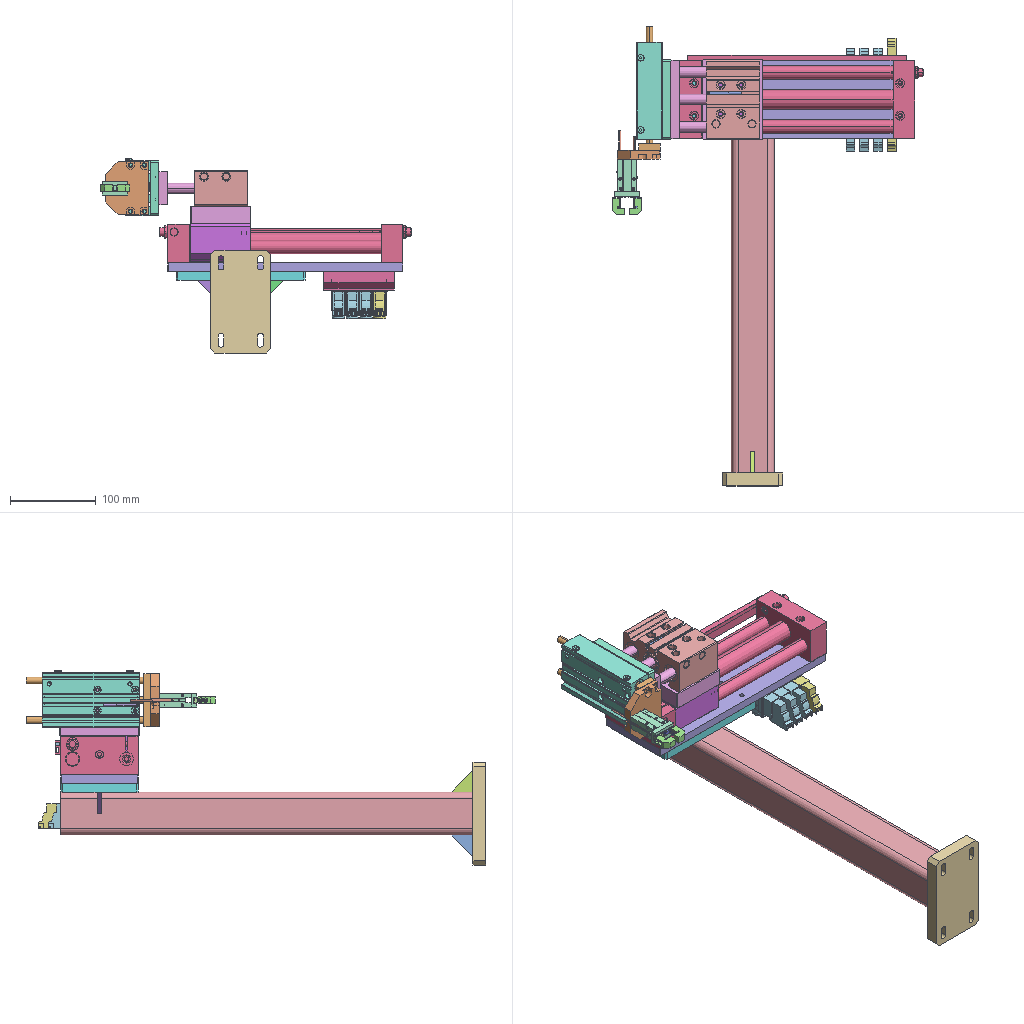Assembly | SolidWorks | 19 different items | 23 placed | box 362 x 536 x 226 mm
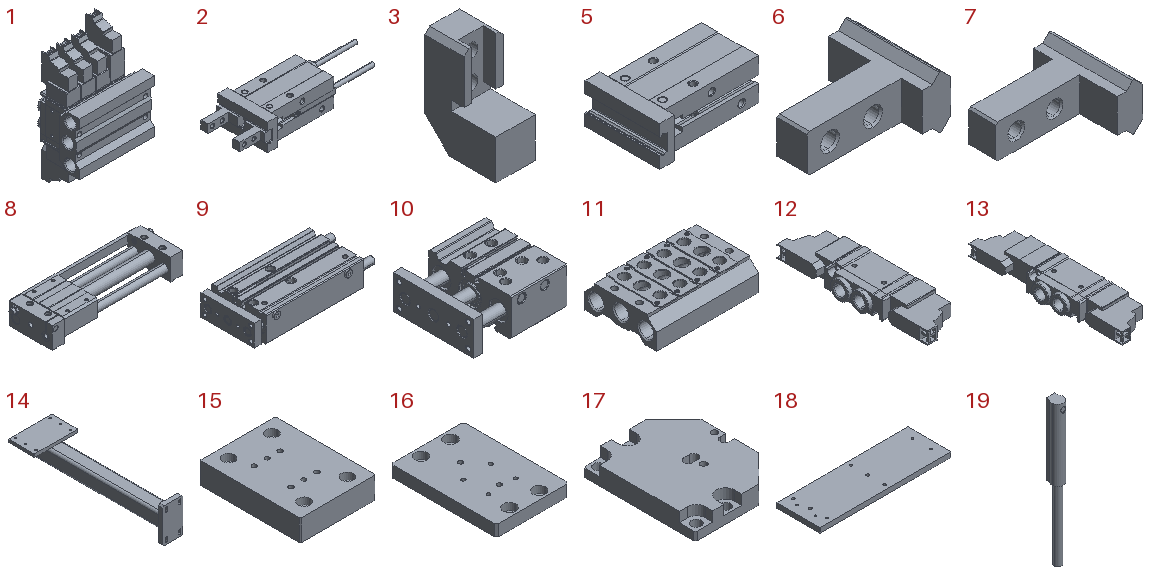Parts list (item | name | quantity | parent item | size | volume | features):
1 | (subassembly) | x1 | - | 82 x 55.3 x 132 mm | 207310 mm3 | -
2 | (subassembly) | x1 | - | 90 x 30 x 16.5 mm | 15703 mm3 | -
3 | - | x2 | - | 8 x 14.5 x 20 mm | 1262 mm3 | features Chamfer 2, ICE 2, Cut 1, Extrusion 1, HoleWzd 1
4 | - | x1 | in 2 | - | - | features MBimport 1
5 | - | x1 | in 2 | 43.5 x 30 x 16.5 mm | 13735 mm3 | features BaseBody 1
6 | - | x1 | in 2 | 16.2 x 12.4 x 6.994 mm | 484.765 mm3 | features BaseBody 1
7 | - | x1 | in 2 | 16.2 x 12.4 x 6.994 mm | 484.765 mm3 | features BaseBody 1
8 | - | x1 | - | 294 x 96.8 x 46 mm | 580391 mm3 | features BaseBody 4, MoveCopyBody 1
9 | - | x1 | - | 145 x 66.1 x 30 mm | 183701 mm3 | features BaseBody 4, MoveCopyBody 1
10 | - | x1 | - | 103.5 x 93 x 42 mm | 225365 mm3 | features BaseBody 4, MoveCopyBody 1
11 | - | x1 | in 1 | 82 x 57.5 x 22.8 mm | 48619 mm3 | features MBimport 1
12 | - | x3 | in 1 | 32.5 x 120 x 16.6 mm | 38659 mm3 | features BaseBody 1
13 | - | x1 | in 1 | 32.5 x 132 x 16.6 mm | 42705 mm3 | features BaseBody 1
14 | - | x1 | - | 150 x 495 x 120 mm | 600253 mm3 | features Gusset 4, HoleWzd 4, Chamfer 2, ICE 2, EndCap 1, WeldMemberFeat 1, WeldmentFeature 1
15 | - | x1 | - | 70 x 93 x 20 mm | 124255 mm3 | features HoleWzd 3, Chamfer 1, Extrusion 1
16 | - | x1 | - | 64 x 93 x 10 mm | 55951 mm3 | features HoleWzd 4, Chamfer 1, Extrusion 1
17 | - | x1 | - | 50 x 62 x 10 mm | 25616 mm3 | features Chamfer 3, HoleWzd 3, ICE 2, Cut 1, Extrusion 1
18 | - | x1 | - | 274 x 90 x 10 mm | 244675 mm3 | features HoleWzd 3, Chamfer 1, Extrusion 1
19 | - | x2 | in 2 | 4 x 5.4 x 50 mm | 499.041 mm3 | features BaseBody 1
Mates (type | each side: item.copy, entity, surface, feature):
In the top assembly
Coincident | 10.1 face plane TC-L-25x2525_b-1-solid1 | 15.1 face plane Boss-Extrude1
Width | 10.1 face plane TC-L-25x2525_b-1-solid1 | 10.1 face plane TC-L-25x2525_b-1-solid1 | 15.1 face plane Boss-Extrude1 | 15.1 face plane Boss-Extrude1
Width | 15.1 face plane Boss-Extrude1 | 15.1 face plane Boss-Extrude1 | 10.1 face plane TC-L-25x2525_b-1-solid1 | 10.1 face plane TC-L-25x2525_b-1-solid1
Coincident | 10.1 face plane TCL-25x25-0_25fp-1-solid1 | 16.1 face plane Boss-Extrude1
Width | 10.1 face plane TCL-25x25-0_25fp-1-solid1 | 10.1 face plane TCL-25x25-0_25fp-1-solid1 | 16.1 face plane Boss-Extrude1 | 16.1 face plane Boss-Extrude1 | 2 times
Coincident | 9.1 face plane TC-L-16x8080_b-1-solid1 | 16.1 face plane Boss-Extrude1 | 2 times
Width | 16.1 face plane Boss-Extrude1 | 16.1 face plane Boss-Extrude1 | 9.1 face plane TC-L-16x8080_b-1-solid1 | 9.1 face plane TC-L-16x8080_b-1-solid1
Coincident | 9.1 face plane TCL-16x80-0_80fp-1-solid1 | 17.1 face plane Boss-Extrude1 | 2 times
Width | 17.1 face plane Boss-Extrude1 | 17.1 face plane Boss-Extrude1 | 9.1 face plane TCL-16x80-0_80fp-1-solid1 | 9.1 face plane TCL-16x80-0_80fp-1-solid1
Coincident | 18.1 face plane Boss-Extrude1 | 14.1 face plane Boss-Extrude2 | 2 times
DistanceDim | 14.1 plane | 18.1 face plane Boss-Extrude1
Coincident | 18.1 face plane Boss-Extrude1 | 8.1 face plane RMT-20X150-S(0)_rod-1-solid1
Width | 18.1 face plane Boss-Extrude1 | 18.1 face plane Boss-Extrude1 | 8.1 face plane RMT-20X150-S(0)_rod-1-solid1 | 8.1 face plane RMT-20X150-S(0)_rod-1-solid1
Width | 8.1 face plane RMT-20X150-S(0)_rod-1-solid1 | 8.1 face plane RMT-20X150-S(0)_rod-1-solid1 | 18.1 face plane Boss-Extrude1 | 18.1 face plane Boss-Extrude1
Coincident | 15.1 face plane Boss-Extrude1 | 8.1 face plane RMT-20X150-S(0)_body-1-solid1
Width | 15.1 face plane Boss-Extrude1 | 15.1 face plane Boss-Extrude1 | 8.1 face plane RMT-20X150-S(0)_body-1-solid1 | 8.1 face plane RMT-20X150-S(0)_body-1-solid1 | 2 times
Coincident | 17.1 face plane Boss-Extrude1 | 5.1 face plane Input1 | 2 times
Width | 17.1 face plane Boss-Extrude1 | 17.1 face plane Boss-Extrude1 | 5.1 face plane Input1 | 5.1 face plane Input1
Coincident | 6.1 face plane Input1 | 3.1 face plane Cut-Extrude1
Concentric | 6.1 face cylinder Input1 | 3.1 face cylinder CBORE for M2.5 Hex Socket Head Cap Screw2
Parallel | 6.1 face plane Input1 | 3.1 face plane Boss-Extrude1
Concentric | 7.1 face cylinder Input1 | 3.2 face cylinder CBORE for M2.5 Hex Socket Head Cap Screw2
Parallel | 7.1 face plane Input1 | 3.2 face plane Boss-Extrude1
Coincident | 7.1 face plane Input1 | 3.2 face plane Cut-Extrude1
Coincident | 18.1 face plane Boss-Extrude1 | 11.1 face plane 7V100M4F.stp<1>
Width | 18.1 face plane Boss-Extrude1 | 18.1 face plane Boss-Extrude1 | 11.1 face plane 7V100M4F.stp<1> | 11.1 face plane 7V100M4F.stp<1>
DistanceDim | 18.1 face plane Boss-Extrude1 | 11.1 face plane 7V100M4F.stp<1>
In subassembly 1
Coincident | 11.2 plane | 1.1 plane | 3 times
Concentric | 11.2 face cylinder 7V100M4F.stp<1> | 12.1 face cylinder Input1 | 2 times
Coincident | 11.2 face plane 7V100M4F.stp<1> | 12.1 face plane Input1
Concentric | 11.2 face cylinder 7V100M4F.stp<1> | 12.2 face cylinder Input1 | 2 times
Coincident | 11.2 face plane 7V100M4F.stp<1> | 12.2 face plane Input1
Concentric | 11.2 face cylinder 7V100M4F.stp<1> | 12.3 face cylinder Input1 | 2 times
Coincident | 11.2 face plane 7V100M4F.stp<1> | 12.3 face plane Input1
Concentric | 11.2 face cylinder 7V100M4F.stp<1> | 13.1 face cylinder Input1 | 2 times
Coincident | 11.2 face plane 7V100M4F.stp<1> | 13.1 face plane Input1
In subassembly 2
DistanceDim | 5.2 face plane Input1 | 6.2 face plane Input1
LimitDistanceDim | 6.2 face plane Input1 | 7.2 face plane Input1
Width | 5.2 face plane Input1 | 5.2 face plane Input1 | 6.2 face plane Input1 | 6.2 face plane Input1
Width | 5.2 face plane Input1 | 5.2 face plane Input1 | 7.2 face plane Input1 | 6.2 face plane Input1
Coincident | 6.2 face plane Input1 | 7.2 face plane Input1 | 2 times